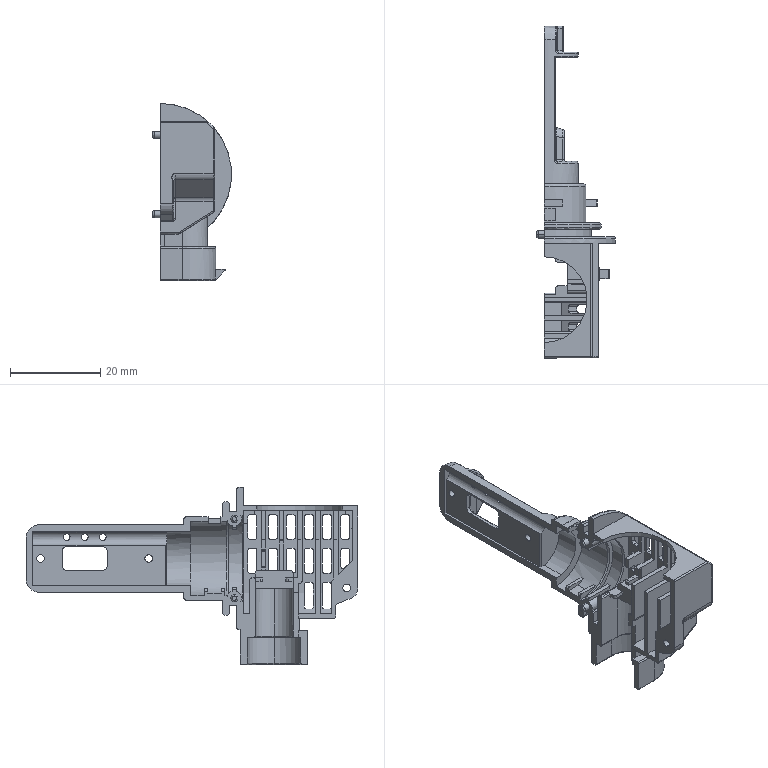Part | SolidWorks | features ICE 9, MoveFace 4, BaseBody 1, Chamfer 1, Fillet 1 | 1 solid | 528 faces | box 17.45 x 73.802 x 39.25 mm | volume 4637 mm3 | plane 239 | cylinder 196 | spline 84 | cone 6 | torus 3 | commonest cylinder face diameters 1 x77 0.6 x68 2 x7 1.5 x6 1.7 x6 1.6 x4